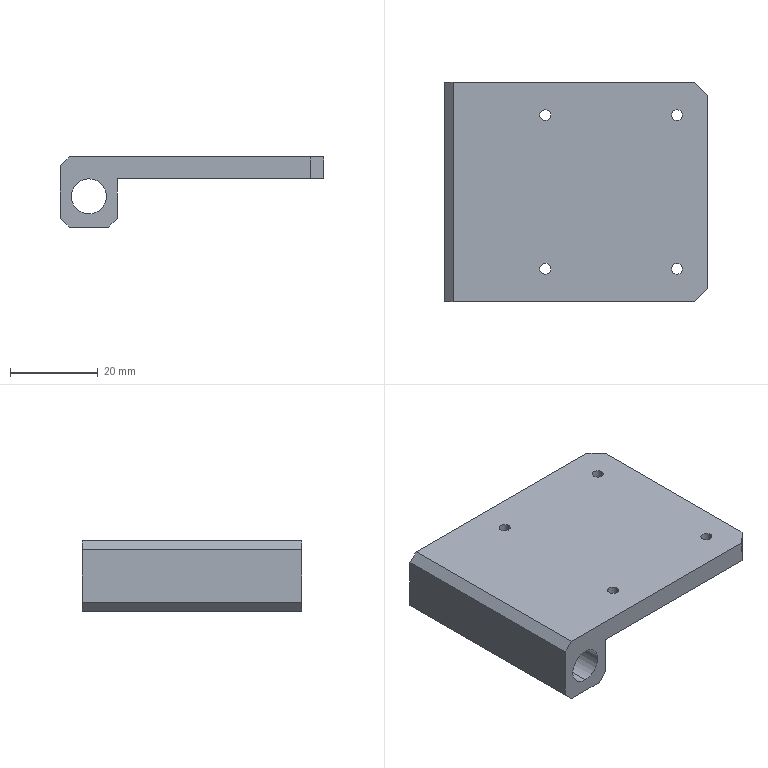Part | SolidWorks | features Chamfer 3, ICE 2, 3DProfileFeature 1, Extrusion 1, HoleWzd 1, LPattern 1 | 1 solid | 31 faces | box 60 x 50 x 16 mm | volume 19181 mm3 | plane 13 | cylinder 10 | cone 8 | commonest cylinder face diameters 2.5 x8 8 x2
STEP:
#1=CARTESIAN_POINT('',(24.25,42.5,-4.2));
#2=VERTEX_POINT('',#1);
#3=CARTESIAN_POINT('',(21.75,42.5,-4.2));
#4=VERTEX_POINT('',#3);
#5=CARTESIAN_POINT('',(23.,42.5,-4.2));
#6=DIRECTION('',(0.,0.,-1.));
#7=DIRECTION('',(1.,0.,0.));
#8=AXIS2_PLACEMENT_3D('',#5,#6,#7);
#9=CIRCLE('',#8,1.25);
#10=EDGE_CURVE('',#2,#4,#9,.T.);
#11=ORIENTED_EDGE('',*,*,#10,.F.);
#12=CARTESIAN_POINT('',(25.05,42.5,-5.));
#13=VERTEX_POINT('',#12);
#14=CARTESIAN_POINT('',(25.05,42.5,-5.));
#15=DIRECTION('',(0.7071,0.,-0.7071));
#16=VECTOR('',#15,1000.);
#17=LINE('',#14,#16);
#18=EDGE_CURVE('',#2,#13,#17,.T.);
#19=ORIENTED_EDGE('',*,*,#18,.T.);
#20=CARTESIAN_POINT('',(20.95,42.5,-5.));
#21=VERTEX_POINT('',#20);
#22=CARTESIAN_POINT('',(23.,42.5,-5.));
#23=DIRECTION('',(0.,0.,1.));
#24=DIRECTION('',(1.,0.,0.));
#25=AXIS2_PLACEMENT_3D('',#22,#23,#24);
#26=CIRCLE('',#25,2.05);
#27=EDGE_CURVE('',#21,#13,#26,.T.);
#28=ORIENTED_EDGE('',*,*,#27,.F.);
#29=CARTESIAN_POINT('',(20.95,42.5,-5.));
#30=DIRECTION('',(-0.7071,0.,-0.7071));
#31=VECTOR('',#30,1000.);
#32=LINE('',#29,#31);
#33=EDGE_CURVE('',#4,#21,#32,.T.);
#34=ORIENTED_EDGE('',*,*,#33,.F.);
#35=EDGE_LOOP('',(#11,#19,#28,#34));
#36=FACE_OUTER_BOUND('',#35,.T.);
#37=CARTESIAN_POINT('',(23.,42.5,-5.));
#38=DIRECTION('',(0.,0.,-1.));
#39=DIRECTION('',(-1.,0.,0.));
#40=AXIS2_PLACEMENT_3D('',#37,#38,#39);
#41=CONICAL_SURFACE('',#40,2.05,0.7854);
#42=ADVANCED_FACE('',(#36),#41,.F.);
#43=CARTESIAN_POINT('',(54.25,42.5,-4.2));
#44=VERTEX_POINT('',#43);
#45=CARTESIAN_POINT('',(51.75,42.5,-4.2));
#46=VERTEX_POINT('',#45);
#47=CARTESIAN_POINT('',(53.,42.5,-4.2));
#48=DIRECTION('',(0.,0.,-1.));
#49=DIRECTION('',(1.,0.,0.));
#50=AXIS2_PLACEMENT_3D('',#47,#48,#49);
#51=CIRCLE('',#50,1.25);
#52=EDGE_CURVE('',#44,#46,#51,.T.);
#53=ORIENTED_EDGE('',*,*,#52,.F.);
#54=CARTESIAN_POINT('',(55.05,42.5,-5.));
#55=VERTEX_POINT('',#54);
#56=CARTESIAN_POINT('',(55.05,42.5,-5.));
#57=DIRECTION('',(0.7071,0.,-0.7071));
#58=VECTOR('',#57,1000.);
#59=LINE('',#56,#58);
#60=EDGE_CURVE('',#44,#55,#59,.T.);
#61=ORIENTED_EDGE('',*,*,#60,.T.);
#62=CARTESIAN_POINT('',(50.95,42.5,-5.));
#63=VERTEX_POINT('',#62);
#64=CARTESIAN_POINT('',(53.,42.5,-5.));
#65=DIRECTION('',(0.,0.,1.));
#66=DIRECTION('',(1.,0.,0.));
#67=AXIS2_PLACEMENT_3D('',#64,#65,#66);
#68=CIRCLE('',#67,2.05);
#69=EDGE_CURVE('',#63,#55,#68,.T.);
#70=ORIENTED_EDGE('',*,*,#69,.F.);
#71=CARTESIAN_POINT('',(50.95,42.5,-5.));
#72=DIRECTION('',(-0.7071,0.,-0.7071));
#73=VECTOR('',#72,1000.);
#74=LINE('',#71,#73);
#75=EDGE_CURVE('',#46,#63,#74,.T.);
#76=ORIENTED_EDGE('',*,*,#75,.F.);
#77=EDGE_LOOP('',(#53,#61,#70,#76));
#78=FACE_OUTER_BOUND('',#77,.T.);
#79=CARTESIAN_POINT('',(53.,42.5,-5.));
#80=DIRECTION('',(0.,0.,-1.));
#81=DIRECTION('',(-1.,0.,0.));
#82=AXIS2_PLACEMENT_3D('',#79,#80,#81);
#83=CONICAL_SURFACE('',#82,2.05,0.7854);
#84=ADVANCED_FACE('',(#78),#83,.F.);
#85=CARTESIAN_POINT('',(24.25,7.5,-4.2));
#86=VERTEX_POINT('',#85);
#87=CARTESIAN_POINT('',(21.75,7.5,-4.2));
#88=VERTEX_POINT('',#87);
#89=CARTESIAN_POINT('',(23.,7.5,-4.2));
#90=DIRECTION('',(0.,0.,-1.));
#91=DIRECTION('',(1.,0.,0.));
#92=AXIS2_PLACEMENT_3D('',#89,#90,#91);
#93=CIRCLE('',#92,1.25);
#94=EDGE_CURVE('',#86,#88,#93,.T.);
#95=ORIENTED_EDGE('',*,*,#94,.F.);
#96=CARTESIAN_POINT('',(25.05,7.5,-5.));
#97=VERTEX_POINT('',#96);
#98=CARTESIAN_POINT('',(25.05,7.5,-5.));
#99=DIRECTION('',(0.7071,0.,-0.7071));
#100=VECTOR('',#99,1000.);
#101=LINE('',#98,#100);
#102=EDGE_CURVE('',#86,#97,#101,.T.);
#103=ORIENTED_EDGE('',*,*,#102,.T.);
#104=CARTESIAN_POINT('',(20.95,7.5,-5.));
#105=VERTEX_POINT('',#104);
#106=CARTESIAN_POINT('',(23.,7.5,-5.));
#107=DIRECTION('',(0.,0.,1.));
#108=DIRECTION('',(1.,0.,0.));
#109=AXIS2_PLACEMENT_3D('',#106,#107,#108);
#110=CIRCLE('',#109,2.05);
#111=EDGE_CURVE('',#105,#97,#110,.T.);
#112=ORIENTED_EDGE('',*,*,#111,.F.);
#113=CARTESIAN_POINT('',(20.95,7.5,-5.));
#114=DIRECTION('',(-0.7071,0.,-0.7071));
#115=VECTOR('',#114,1000.);
#116=LINE('',#113,#115);
#117=EDGE_CURVE('',#88,#105,#116,.T.);
#118=ORIENTED_EDGE('',*,*,#117,.F.);
#119=EDGE_LOOP('',(#95,#103,#112,#118));
#120=FACE_OUTER_BOUND('',#119,.T.);
#121=CARTESIAN_POINT('',(23.,7.5,-5.));
#122=DIRECTION('',(0.,0.,-1.));
#123=DIRECTION('',(-1.,0.,0.));
#124=AXIS2_PLACEMENT_3D('',#121,#122,#123);
#125=CONICAL_SURFACE('',#124,2.05,0.7854);
#126=ADVANCED_FACE('',(#120),#125,.F.);
#127=CARTESIAN_POINT('',(54.25,7.5,-4.2));
#128=VERTEX_POINT('',#127);
#129=CARTESIAN_POINT('',(51.75,7.5,-4.2));
#130=VERTEX_POINT('',#129);
#131=CARTESIAN_POINT('',(53.,7.5,-4.2));
#132=DIRECTION('',(0.,0.,-1.));
#133=DIRECTION('',(1.,0.,0.));
#134=AXIS2_PLACEMENT_3D('',#131,#132,#133);
#135=CIRCLE('',#134,1.25);
#136=EDGE_CURVE('',#128,#130,#135,.T.);
#137=ORIENTED_EDGE('',*,*,#136,.F.);
#138=CARTESIAN_POINT('',(55.05,7.5,-5.));
#139=VERTEX_POINT('',#138);
#140=CARTESIAN_POINT('',(55.05,7.5,-5.));
#141=DIRECTION('',(0.7071,0.,-0.7071));
#142=VECTOR('',#141,1000.);
#143=LINE('',#140,#142);
#144=EDGE_CURVE('',#128,#139,#143,.T.);
#145=ORIENTED_EDGE('',*,*,#144,.T.);
#146=CARTESIAN_POINT('',(50.95,7.5,-5.));
#147=VERTEX_POINT('',#146);
#148=CARTESIAN_POINT('',(53.,7.5,-5.));
#149=DIRECTION('',(0.,0.,1.));
#150=DIRECTION('',(1.,0.,0.));
#151=AXIS2_PLACEMENT_3D('',#148,#149,#150);
#152=CIRCLE('',#151,2.05);
#153=EDGE_CURVE('',#147,#139,#152,.T.);
#154=ORIENTED_EDGE('',*,*,#153,.F.);
#155=CARTESIAN_POINT('',(50.95,7.5,-5.));
#156=DIRECTION('',(-0.7071,0.,-0.7071));
#157=VECTOR('',#156,1000.);
#158=LINE('',#155,#157);
#159=EDGE_CURVE('',#130,#147,#158,.T.);
#160=ORIENTED_EDGE('',*,*,#159,.F.);
#161=EDGE_LOOP('',(#137,#145,#154,#160));
#162=FACE_OUTER_BOUND('',#161,.T.);
#163=CARTESIAN_POINT('',(53.,7.5,-5.));
#164=DIRECTION('',(0.,0.,-1.));
#165=DIRECTION('',(-1.,0.,0.));
#166=AXIS2_PLACEMENT_3D('',#163,#164,#165);
#167=CONICAL_SURFACE('',#166,2.05,0.7854);
#168=ADVANCED_FACE('',(#162),#167,.F.);
#169=ORIENTED_EDGE('',*,*,#10,.T.);
#170=CARTESIAN_POINT('',(21.75,42.5,0.));
#171=VERTEX_POINT('',#170);
#172=CARTESIAN_POINT('',(21.75,42.5,0.));
#173=DIRECTION('',(0.,0.,1.));
#174=VECTOR('',#173,1000.);
#175=LINE('',#172,#174);
#176=EDGE_CURVE('',#4,#171,#175,.T.);
#177=ORIENTED_EDGE('',*,*,#176,.T.);
#178=CARTESIAN_POINT('',(24.25,42.5,0.));
#179=VERTEX_POINT('',#178);
#180=CARTESIAN_POINT('',(23.,42.5,0.));
#181=DIRECTION('',(0.,0.,1.));
#182=DIRECTION('',(1.,0.,0.));
#183=AXIS2_PLACEMENT_3D('',#180,#181,#182);
#184=CIRCLE('',#183,1.25);
#185=EDGE_CURVE('',#171,#179,#184,.T.);
#186=ORIENTED_EDGE('',*,*,#185,.T.);
#187=CARTESIAN_POINT('',(24.25,42.5,0.));
#188=DIRECTION('',(0.,0.,1.));
#189=VECTOR('',#188,1000.);
#190=LINE('',#187,#189);
#191=EDGE_CURVE('',#2,#179,#190,.T.);
#192=ORIENTED_EDGE('',*,*,#191,.F.);
#193=EDGE_LOOP('',(#169,#177,#186,#192));
#194=FACE_OUTER_BOUND('',#193,.T.);
#195=CARTESIAN_POINT('',(23.,42.5,0.));
#196=DIRECTION('',(0.,0.,1.));
#197=DIRECTION('',(1.,0.,0.));
#198=AXIS2_PLACEMENT_3D('',#195,#196,#197);
#199=CYLINDRICAL_SURFACE('',#198,1.25);
#200=ADVANCED_FACE('',(#194),#199,.F.);
#201=ORIENTED_EDGE('',*,*,#52,.T.);
#202=CARTESIAN_POINT('',(51.75,42.5,0.));
#203=VERTEX_POINT('',#202);
#204=CARTESIAN_POINT('',(51.75,42.5,0.));
#205=DIRECTION('',(0.,0.,1.));
#206=VECTOR('',#205,1000.);
#207=LINE('',#204,#206);
#208=EDGE_CURVE('',#46,#203,#207,.T.);
#209=ORIENTED_EDGE('',*,*,#208,.T.);
#210=CARTESIAN_POINT('',(54.25,42.5,0.));
#211=VERTEX_POINT('',#210);
#212=CARTESIAN_POINT('',(53.,42.5,0.));
#213=DIRECTION('',(0.,0.,1.));
#214=DIRECTION('',(1.,0.,0.));
#215=AXIS2_PLACEMENT_3D('',#212,#213,#214);
#216=CIRCLE('',#215,1.25);
#217=EDGE_CURVE('',#203,#211,#216,.T.);
#218=ORIENTED_EDGE('',*,*,#217,.T.);
#219=CARTESIAN_POINT('',(54.25,42.5,0.));
#220=DIRECTION('',(0.,0.,1.));
#221=VECTOR('',#220,1000.);
#222=LINE('',#219,#221);
#223=EDGE_CURVE('',#44,#211,#222,.T.);
#224=ORIENTED_EDGE('',*,*,#223,.F.);
#225=EDGE_LOOP('',(#201,#209,#218,#224));
#226=FACE_OUTER_BOUND('',#225,.T.);
#227=CARTESIAN_POINT('',(53.,42.5,0.));
#228=DIRECTION('',(0.,0.,1.));
#229=DIRECTION('',(1.,0.,0.));
#230=AXIS2_PLACEMENT_3D('',#227,#228,#229);
#231=CYLINDRICAL_SURFACE('',#230,1.25);
#232=ADVANCED_FACE('',(#226),#231,.F.);
#233=ORIENTED_EDGE('',*,*,#136,.T.);
#234=CARTESIAN_POINT('',(51.75,7.5,0.));
#235=VERTEX_POINT('',#234);
#236=CARTESIAN_POINT('',(51.75,7.5,0.));
#237=DIRECTION('',(0.,0.,1.));
#238=VECTOR('',#237,1000.);
#239=LINE('',#236,#238);
#240=EDGE_CURVE('',#130,#235,#239,.T.);
#241=ORIENTED_EDGE('',*,*,#240,.T.);
#242=CARTESIAN_POINT('',(54.25,7.5,0.));
#243=VERTEX_POINT('',#242);
#244=CARTESIAN_POINT('',(53.,7.5,0.));
#245=DIRECTION('',(0.,0.,1.));
#246=DIRECTION('',(1.,0.,0.));
#247=AXIS2_PLACEMENT_3D('',#244,#245,#246);
#248=CIRCLE('',#247,1.25);
#249=EDGE_CURVE('',#235,#243,#248,.T.);
#250=ORIENTED_EDGE('',*,*,#249,.T.);
#251=CARTESIAN_POINT('',(54.25,7.5,0.));
#252=DIRECTION('',(0.,0.,1.));
#253=VECTOR('',#252,1000.);
#254=LINE('',#251,#253);
#255=EDGE_CURVE('',#128,#243,#254,.T.);
#256=ORIENTED_EDGE('',*,*,#255,.F.);
#257=EDGE_LOOP('',(#233,#241,#250,#256));
#258=FACE_OUTER_BOUND('',#257,.T.);
#259=CARTESIAN_POINT('',(53.,7.5,0.));
#260=DIRECTION('',(0.,0.,1.));
#261=DIRECTION('',(1.,0.,0.));
#262=AXIS2_PLACEMENT_3D('',#259,#260,#261);
#263=CYLINDRICAL_SURFACE('',#262,1.25);
#264=ADVANCED_FACE('',(#258),#263,.F.);
#265=ORIENTED_EDGE('',*,*,#94,.T.);
#266=CARTESIAN_POINT('',(21.75,7.5,0.));
#267=VERTEX_POINT('',#266);
#268=CARTESIAN_POINT('',(21.75,7.5,0.));
#269=DIRECTION('',(0.,0.,1.));
#270=VECTOR('',#269,1000.);
#271=LINE('',#268,#270);
#272=EDGE_CURVE('',#88,#267,#271,.T.);
#273=ORIENTED_EDGE('',*,*,#272,.T.);
#274=CARTESIAN_POINT('',(24.25,7.5,0.));
#275=VERTEX_POINT('',#274);
#276=CARTESIAN_POINT('',(23.,7.5,0.));
#277=DIRECTION('',(0.,0.,1.));
#278=DIRECTION('',(1.,0.,0.));
#279=AXIS2_PLACEMENT_3D('',#276,#277,#278);
#280=CIRCLE('',#279,1.25);
#281=EDGE_CURVE('',#267,#275,#280,.T.);
#282=ORIENTED_EDGE('',*,*,#281,.T.);
#283=CARTESIAN_POINT('',(24.25,7.5,0.));
#284=DIRECTION('',(0.,0.,1.));
#285=VECTOR('',#284,1000.);
#286=LINE('',#283,#285);
#287=EDGE_CURVE('',#86,#275,#286,.T.);
#288=ORIENTED_EDGE('',*,*,#287,.F.);
#289=EDGE_LOOP('',(#265,#273,#282,#288));
#290=FACE_OUTER_BOUND('',#289,.T.);
#291=CARTESIAN_POINT('',(23.,7.5,0.));
#292=DIRECTION('',(0.,0.,1.));
#293=DIRECTION('',(1.,0.,0.));
#294=AXIS2_PLACEMENT_3D('',#291,#292,#293);
#295=CYLINDRICAL_SURFACE('',#294,1.25);
#296=ADVANCED_FACE('',(#290),#295,.F.);
#297=CARTESIAN_POINT('',(6.5,0.,-5.));
#298=VERTEX_POINT('',#297);
#299=CARTESIAN_POINT('',(6.5,0.,-13.));
#300=VERTEX_POINT('',#299);
#301=CARTESIAN_POINT('',(6.5,0.,-9.));
#302=DIRECTION('',(0.,-1.,0.));
#303=DIRECTION('',(0.,0.,-1.));
#304=AXIS2_PLACEMENT_3D('',#301,#302,#303);
#305=CIRCLE('',#304,4.);
#306=EDGE_CURVE('',#298,#300,#305,.T.);
#307=ORIENTED_EDGE('',*,*,#306,.T.);
#308=CARTESIAN_POINT('',(6.5,50.,-13.));
#309=VERTEX_POINT('',#308);
#310=CARTESIAN_POINT('',(6.5,-10.,-13.));
#311=DIRECTION('',(0.,1.,0.));
#312=VECTOR('',#311,1000.);
#313=LINE('',#310,#312);
#314=EDGE_CURVE('',#300,#309,#313,.T.);
#315=ORIENTED_EDGE('',*,*,#314,.T.);
#316=CARTESIAN_POINT('',(6.5,50.,-5.));
#317=VERTEX_POINT('',#316);
#318=CARTESIAN_POINT('',(6.5,50.,-9.));
#319=DIRECTION('',(0.,1.,0.));
#320=DIRECTION('',(0.,0.,1.));
#321=AXIS2_PLACEMENT_3D('',#318,#319,#320);
#322=CIRCLE('',#321,4.);
#323=EDGE_CURVE('',#309,#317,#322,.T.);
#324=ORIENTED_EDGE('',*,*,#323,.T.);
#325=CARTESIAN_POINT('',(6.5,-10.,-5.));
#326=DIRECTION('',(0.,1.,0.));
#327=VECTOR('',#326,1000.);
#328=LINE('',#325,#327);
#329=EDGE_CURVE('',#298,#317,#328,.T.);
#330=ORIENTED_EDGE('',*,*,#329,.F.);
#331=EDGE_LOOP('',(#307,#315,#324,#330));
#332=FACE_OUTER_BOUND('',#331,.T.);
#333=CARTESIAN_POINT('',(6.5,-10.,-9.));
#334=DIRECTION('',(0.,1.,0.));
#335=DIRECTION('',(0.,0.,1.));
#336=AXIS2_PLACEMENT_3D('',#333,#334,#335);
#337=CYLINDRICAL_SURFACE('',#336,4.);
#338=ADVANCED_FACE('',(#332),#337,.F.);
#339=CARTESIAN_POINT('',(0.,0.,-14.));
#340=VERTEX_POINT('',#339);
#341=CARTESIAN_POINT('',(0.,0.,-2.));
#342=VERTEX_POINT('',#341);
#343=CARTESIAN_POINT('',(0.,0.,0.));
#344=DIRECTION('',(0.,0.,1.));
#345=VECTOR('',#344,1000.);
#346=LINE('',#343,#345);
#347=EDGE_CURVE('',#340,#342,#346,.T.);
#348=ORIENTED_EDGE('',*,*,#347,.T.);
#349=CARTESIAN_POINT('',(0.,50.,-2.));
#350=VERTEX_POINT('',#349);
#351=CARTESIAN_POINT('',(0.,50.,-2.));
#352=DIRECTION('',(0.,1.,0.));
#353=VECTOR('',#352,1000.);
#354=LINE('',#351,#353);
#355=EDGE_CURVE('',#342,#350,#354,.T.);
#356=ORIENTED_EDGE('',*,*,#355,.T.);
#357=CARTESIAN_POINT('',(0.,50.,-14.));
#358=VERTEX_POINT('',#357);
#359=CARTESIAN_POINT('',(0.,50.,0.));
#360=DIRECTION('',(0.,0.,1.));
#361=VECTOR('',#360,1000.);
#362=LINE('',#359,#361);
#363=EDGE_CURVE('',#358,#350,#362,.T.);
#364=ORIENTED_EDGE('',*,*,#363,.F.);
#365=CARTESIAN_POINT('',(0.,50.,-14.));
#366=DIRECTION('',(0.,-1.,0.));
#367=VECTOR('',#366,1000.);
#368=LINE('',#365,#367);
#369=EDGE_CURVE('',#358,#340,#368,.T.);
#370=ORIENTED_EDGE('',*,*,#369,.T.);
#371=EDGE_LOOP('',(#348,#356,#364,#370));
#372=FACE_OUTER_BOUND('',#371,.T.);
#373=CARTESIAN_POINT('',(0.,50.,0.));
#374=DIRECTION('',(1.,0.,0.));
#375=DIRECTION('',(0.,0.,-1.));
#376=AXIS2_PLACEMENT_3D('',#373,#374,#375);
#377=PLANE('',#376);
#378=ADVANCED_FACE('',(#372),#377,.F.);
#379=CARTESIAN_POINT('',(23.,42.5,0.));
#380=DIRECTION('',(0.,0.,1.));
#381=DIRECTION('',(1.,0.,0.));
#382=AXIS2_PLACEMENT_3D('',#379,#380,#381);
#383=CIRCLE('',#382,1.25);
#384=EDGE_CURVE('',#179,#171,#383,.T.);
#385=ORIENTED_EDGE('',*,*,#384,.F.);
#386=ORIENTED_EDGE('',*,*,#185,.F.);
#387=EDGE_LOOP('',(#385,#386));
#388=FACE_BOUND('',#387,.T.);
#389=CARTESIAN_POINT('',(53.,42.5,0.));
#390=DIRECTION('',(0.,0.,1.));
#391=DIRECTION('',(1.,0.,0.));
#392=AXIS2_PLACEMENT_3D('',#389,#390,#391);
#393=CIRCLE('',#392,1.25);
#394=EDGE_CURVE('',#211,#203,#393,.T.);
#395=ORIENTED_EDGE('',*,*,#394,.F.);
#396=ORIENTED_EDGE('',*,*,#217,.F.);
#397=EDGE_LOOP('',(#395,#396));
#398=FACE_BOUND('',#397,.T.);
#399=CARTESIAN_POINT('',(53.,7.5,0.));
#400=DIRECTION('',(0.,0.,1.));
#401=DIRECTION('',(1.,0.,0.));
#402=AXIS2_PLACEMENT_3D('',#399,#400,#401);
#403=CIRCLE('',#402,1.25);
#404=EDGE_CURVE('',#243,#235,#403,.T.);
#405=ORIENTED_EDGE('',*,*,#404,.F.);
#406=ORIENTED_EDGE('',*,*,#249,.F.);
#407=EDGE_LOOP('',(#405,#406));
#408=FACE_BOUND('',#407,.T.);
#409=CARTESIAN_POINT('',(23.,7.5,0.));
#410=DIRECTION('',(0.,0.,1.));
#411=DIRECTION('',(1.,0.,0.));
#412=AXIS2_PLACEMENT_3D('',#409,#410,#411);
#413=CIRCLE('',#412,1.25);
#414=EDGE_CURVE('',#275,#267,#413,.T.);
#415=ORIENTED_EDGE('',*,*,#414,.F.);
#416=ORIENTED_EDGE('',*,*,#281,.F.);
#417=EDGE_LOOP('',(#415,#416));
#418=FACE_BOUND('',#417,.T.);
#419=CARTESIAN_POINT('',(2.,0.,0.));
#420=VERTEX_POINT('',#419);
#421=CARTESIAN_POINT('',(57.,0.,0.));
#422=VERTEX_POINT('',#421);
#423=CARTESIAN_POINT('',(0.,0.,0.));
#424=DIRECTION('',(1.,0.,0.));
#425=VECTOR('',#424,1000.);
#426=LINE('',#423,#425);
#427=EDGE_CURVE('',#420,#422,#426,.T.);
#428=ORIENTED_EDGE('',*,*,#427,.T.);
#429=CARTESIAN_POINT('',(60.,3.,0.));
#430=VERTEX_POINT('',#429);
#431=CARTESIAN_POINT('',(60.,3.,0.));
#432=DIRECTION('',(0.7071,0.7071,0.));
#433=VECTOR('',#432,1000.);
#434=LINE('',#431,#433);
#435=EDGE_CURVE('',#422,#430,#434,.T.);
#436=ORIENTED_EDGE('',*,*,#435,.T.);
#437=CARTESIAN_POINT('',(60.,47.,0.));
#438=VERTEX_POINT('',#437);
#439=CARTESIAN_POINT('',(60.,50.,0.));
#440=DIRECTION('',(0.,-1.,0.));
#441=VECTOR('',#440,1000.);
#442=LINE('',#439,#441);
#443=EDGE_CURVE('',#438,#430,#442,.T.);
#444=ORIENTED_EDGE('',*,*,#443,.F.);
#445=CARTESIAN_POINT('',(57.,50.,0.));
#446=VERTEX_POINT('',#445);
#447=CARTESIAN_POINT('',(57.,50.,0.));
#448=DIRECTION('',(-0.7071,0.7071,0.));
#449=VECTOR('',#448,1000.);
#450=LINE('',#447,#449);
#451=EDGE_CURVE('',#438,#446,#450,.T.);
#452=ORIENTED_EDGE('',*,*,#451,.T.);
#453=CARTESIAN_POINT('',(2.,50.,0.));
#454=VERTEX_POINT('',#453);
#455=CARTESIAN_POINT('',(0.,50.,0.));
#456=DIRECTION('',(1.,0.,0.));
#457=VECTOR('',#456,1000.);
#458=LINE('',#455,#457);
#459=EDGE_CURVE('',#454,#446,#458,.T.);
#460=ORIENTED_EDGE('',*,*,#459,.F.);
#461=CARTESIAN_POINT('',(2.,50.,0.));
#462=DIRECTION('',(0.,-1.,0.));
#463=VECTOR('',#462,1000.);
#464=LINE('',#461,#463);
#465=EDGE_CURVE('',#454,#420,#464,.T.);
#466=ORIENTED_EDGE('',*,*,#465,.T.);
#467=EDGE_LOOP('',(#428,#436,#444,#452,#460,#466));
#468=FACE_OUTER_BOUND('',#467,.T.);
#469=CARTESIAN_POINT('',(0.,50.,0.));
#470=DIRECTION('',(0.,0.,-1.));
#471=DIRECTION('',(-1.,0.,0.));
#472=AXIS2_PLACEMENT_3D('',#469,#470,#471);
#473=PLANE('',#472);
#474=ADVANCED_FACE('',(#388,#398,#408,#418,#468),#473,.F.);
#475=ORIENTED_EDGE('',*,*,#443,.T.);
#476=CARTESIAN_POINT('',(60.,3.,-5.));
#477=VERTEX_POINT('',#476);
#478=CARTESIAN_POINT('',(60.,3.,-5.));
#479=DIRECTION('',(0.,0.,-1.));
#480=VECTOR('',#479,1000.);
#481=LINE('',#478,#480);
#482=EDGE_CURVE('',#430,#477,#481,.T.);
#483=ORIENTED_EDGE('',*,*,#482,.T.);
#484=CARTESIAN_POINT('',(60.,47.,-5.));
#485=VERTEX_POINT('',#484);
#486=CARTESIAN_POINT('',(60.,50.,-5.));
#487=DIRECTION('',(0.,-1.,0.));
#488=VECTOR('',#487,1000.);
#489=LINE('',#486,#488);
#490=EDGE_CURVE('',#485,#477,#489,.T.);
#491=ORIENTED_EDGE('',*,*,#490,.F.);
#492=CARTESIAN_POINT('',(60.,47.,0.));
#493=DIRECTION('',(0.,0.,1.));
#494=VECTOR('',#493,1000.);
#495=LINE('',#492,#494);
#496=EDGE_CURVE('',#485,#438,#495,.T.);
#497=ORIENTED_EDGE('',*,*,#496,.T.);
#498=EDGE_LOOP('',(#475,#483,#491,#497));
#499=FACE_OUTER_BOUND('',#498,.T.);
#500=CARTESIAN_POINT('',(60.,50.,0.));
#501=DIRECTION('',(-1.,0.,0.));
#502=DIRECTION('',(0.,0.,1.));
#503=AXIS2_PLACEMENT_3D('',#500,#501,#502);
#504=PLANE('',#503);
#505=ADVANCED_FACE('',(#499),#504,.F.);
#506=ORIENTED_EDGE('',*,*,#153,.T.);
#507=CARTESIAN_POINT('',(53.,7.5,-5.));
#508=DIRECTION('',(0.,0.,1.));
#509=DIRECTION('',(1.,0.,0.));
#510=AXIS2_PLACEMENT_3D('',#507,#508,#509);
#511=CIRCLE('',#510,2.05);
#512=EDGE_CURVE('',#139,#147,#511,.T.);
#513=ORIENTED_EDGE('',*,*,#512,.T.);
#514=EDGE_LOOP('',(#506,#513));
#515=FACE_BOUND('',#514,.T.);
#516=ORIENTED_EDGE('',*,*,#111,.T.);
#517=CARTESIAN_POINT('',(23.,7.5,-5.));
#518=DIRECTION('',(0.,0.,1.));
#519=DIRECTION('',(1.,0.,0.));
#520=AXIS2_PLACEMENT_3D('',#517,#518,#519);
#521=CIRCLE('',#520,2.05);
#522=EDGE_CURVE('',#97,#105,#521,.T.);
#523=ORIENTED_EDGE('',*,*,#522,.T.);
#524=EDGE_LOOP('',(#516,#523));
#525=FACE_BOUND('',#524,.T.);
#526=ORIENTED_EDGE('',*,*,#69,.T.);
#527=CARTESIAN_POINT('',(53.,42.5,-5.));
#528=DIRECTION('',(0.,0.,1.));
#529=DIRECTION('',(1.,0.,0.));
#530=AXIS2_PLACEMENT_3D('',#527,#528,#529);
#531=CIRCLE('',#530,2.05);
#532=EDGE_CURVE('',#55,#63,#531,.T.);
#533=ORIENTED_EDGE('',*,*,#532,.T.);
#534=EDGE_LOOP('',(#526,#533));
#535=FACE_BOUND('',#534,.T.);
#536=ORIENTED_EDGE('',*,*,#27,.T.);
#537=CARTESIAN_POINT('',(23.,42.5,-5.));
#538=DIRECTION('',(0.,0.,1.));
#539=DIRECTION('',(1.,0.,0.));
#540=AXIS2_PLACEMENT_3D('',#537,#538,#539);
#541=CIRCLE('',#540,2.05);
#542=EDGE_CURVE('',#13,#21,#541,.T.);
#543=ORIENTED_EDGE('',*,*,#542,.T.);
#544=EDGE_LOOP('',(#536,#543));
#545=FACE_BOUND('',#544,.T.);
#546=ORIENTED_EDGE('',*,*,#490,.T.);
#547=CARTESIAN_POINT('',(57.,0.,-5.));
#548=VERTEX_POINT('',#547);
#549=CARTESIAN_POINT('',(60.,3.,-5.));
#550=DIRECTION('',(-0.7071,-0.7071,0.));
#551=VECTOR('',#550,1000.);
#552=LINE('',#549,#551);
#553=EDGE_CURVE('',#477,#548,#552,.T.);
#554=ORIENTED_EDGE('',*,*,#553,.T.);
#555=CARTESIAN_POINT('',(13.,0.,-5.));
#556=VERTEX_POINT('',#555);
#557=CARTESIAN_POINT('',(60.,0.,-5.));
#558=DIRECTION('',(-1.,0.,0.));
#559=VECTOR('',#558,1000.);
#560=LINE('',#557,#559);
#561=EDGE_CURVE('',#548,#556,#560,.T.);
#562=ORIENTED_EDGE('',*,*,#561,.T.);
#563=CARTESIAN_POINT('',(13.,50.,-5.));
#564=VERTEX_POINT('',#563);
#565=CARTESIAN_POINT('',(13.,50.,-5.));
#566=DIRECTION('',(0.,-1.,0.));
#567=VECTOR('',#566,1000.);
#568=LINE('',#565,#567);
#569=EDGE_CURVE('',#564,#556,#568,.T.);
#570=ORIENTED_EDGE('',*,*,#569,.F.);
#571=CARTESIAN_POINT('',(57.,50.,-5.));
#572=VERTEX_POINT('',#571);
#573=CARTESIAN_POINT('',(60.,50.,-5.));
#574=DIRECTION('',(-1.,0.,0.));
#575=VECTOR('',#574,1000.);
#576=LINE('',#573,#575);
#577=EDGE_CURVE('',#572,#564,#576,.T.);
#578=ORIENTED_EDGE('',*,*,#577,.F.);
#579=CARTESIAN_POINT('',(57.,50.,-5.));
#580=DIRECTION('',(0.7071,-0.7071,0.));
#581=VECTOR('',#580,1000.);
#582=LINE('',#579,#581);
#583=EDGE_CURVE('',#572,#485,#582,.T.);
#584=ORIENTED_EDGE('',*,*,#583,.T.);
#585=EDGE_LOOP('',(#546,#554,#562,#570,#578,#584));
#586=FACE_OUTER_BOUND('',#585,.T.);
#587=CARTESIAN_POINT('',(60.,50.,-5.));
#588=DIRECTION('',(0.,0.,1.));
#589=DIRECTION('',(1.,0.,0.));
#590=AXIS2_PLACEMENT_3D('',#587,#588,#589);
#591=PLANE('',#590);
#592=ADVANCED_FACE('',(#515,#525,#535,#545,#586),#591,.F.);
#593=CARTESIAN_POINT('',(13.,0.,-14.));
#594=VERTEX_POINT('',#593);
#595=CARTESIAN_POINT('',(13.,0.,-16.));
#596=DIRECTION('',(0.,0.,-1.));
#597=VECTOR('',#596,1000.);
#598=LINE('',#595,#597);
#599=EDGE_CURVE('',#556,#594,#598,.T.);
#600=ORIENTED_EDGE('',*,*,#599,.T.);
#601=CARTESIAN_POINT('',(13.,50.,-14.));
#602=VERTEX_POINT('',#601);
#603=CARTESIAN_POINT('',(13.,50.,-14.));
#604=DIRECTION('',(0.,1.,0.));
#605=VECTOR('',#604,1000.);
#606=LINE('',#603,#605);
#607=EDGE_CURVE('',#594,#602,#606,.T.);
#608=ORIENTED_EDGE('',*,*,#607,.T.);
#609=CARTESIAN_POINT('',(13.,50.,-16.));
#610=DIRECTION('',(0.,0.,-1.));
#611=VECTOR('',#610,1000.);
#612=LINE('',#609,#611);
#613=EDGE_CURVE('',#564,#602,#612,.T.);
#614=ORIENTED_EDGE('',*,*,#613,.F.);
#615=ORIENTED_EDGE('',*,*,#569,.T.);
#616=EDGE_LOOP('',(#600,#608,#614,#615));
#617=FACE_OUTER_BOUND('',#616,.T.);
#618=CARTESIAN_POINT('',(13.,50.,-16.));
#619=DIRECTION('',(-1.,0.,0.));
#620=DIRECTION('',(0.,0.,1.));
#621=AXIS2_PLACEMENT_3D('',#618,#619,#620);
#622=PLANE('',#621);
#623=ADVANCED_FACE('',(#617),#622,.F.);
#624=CARTESIAN_POINT('',(11.,0.,-16.));
#625=VERTEX_POINT('',#624);
#626=CARTESIAN_POINT('',(2.,0.,-16.));
#627=VERTEX_POINT('',#626);
#628=CARTESIAN_POINT('',(0.,0.,-16.));
#629=DIRECTION('',(-1.,0.,0.));
#630=VECTOR('',#629,1000.);
#631=LINE('',#628,#630);
#632=EDGE_CURVE('',#625,#627,#631,.T.);
#633=ORIENTED_EDGE('',*,*,#632,.T.);
#634=CARTESIAN_POINT('',(2.,50.,-16.));
#635=VERTEX_POINT('',#634);
#636=CARTESIAN_POINT('',(2.,50.,-16.));
#637=DIRECTION('',(0.,1.,0.));
#638=VECTOR('',#637,1000.);
#639=LINE('',#636,#638);
#640=EDGE_CURVE('',#627,#635,#639,.T.);
#641=ORIENTED_EDGE('',*,*,#640,.T.);
#642=CARTESIAN_POINT('',(11.,50.,-16.));
#643=VERTEX_POINT('',#642);
#644=CARTESIAN_POINT('',(0.,50.,-16.));
#645=DIRECTION('',(-1.,0.,0.));
#646=VECTOR('',#645,1000.);
#647=LINE('',#644,#646);
#648=EDGE_CURVE('',#643,#635,#647,.T.);
#649=ORIENTED_EDGE('',*,*,#648,.F.);
#650=CARTESIAN_POINT('',(11.,50.,-16.));
#651=DIRECTION('',(0.,-1.,0.));
#652=VECTOR('',#651,1000.);
#653=LINE('',#650,#652);
#654=EDGE_CURVE('',#643,#625,#653,.T.);
#655=ORIENTED_EDGE('',*,*,#654,.T.);
#656=EDGE_LOOP('',(#633,#641,#649,#655));
#657=FACE_OUTER_BOUND('',#656,.T.);
#658=CARTESIAN_POINT('',(0.,50.,-16.));
#659=DIRECTION('',(0.,0.,1.));
#660=DIRECTION('',(1.,0.,0.));
#661=AXIS2_PLACEMENT_3D('',#658,#659,#660);
#662=PLANE('',#661);
#663=ADVANCED_FACE('',(#657),#662,.F.);
#664=CARTESIAN_POINT('',(6.5,50.,-9.));
#665=DIRECTION('',(0.,1.,0.));
#666=DIRECTION('',(0.,0.,1.));
#667=AXIS2_PLACEMENT_3D('',#664,#665,#666);
#668=CIRCLE('',#667,4.);
#669=EDGE_CURVE('',#317,#309,#668,.T.);
#670=ORIENTED_EDGE('',*,*,#669,.F.);
#671=ORIENTED_EDGE('',*,*,#323,.F.);
#672=EDGE_LOOP('',(#670,#671));
#673=FACE_BOUND('',#672,.T.);
#674=ORIENTED_EDGE('',*,*,#459,.T.);
#675=CARTESIAN_POINT('',(57.,50.,0.));
#676=DIRECTION('',(0.,0.,-1.));
#677=VECTOR('',#676,1000.);
#678=LINE('',#675,#677);
#679=EDGE_CURVE('',#446,#572,#678,.T.);
#680=ORIENTED_EDGE('',*,*,#679,.T.);
#681=ORIENTED_EDGE('',*,*,#577,.T.);
#682=ORIENTED_EDGE('',*,*,#613,.T.);
#683=CARTESIAN_POINT('',(11.,50.,-16.));
#684=DIRECTION('',(-0.7071,0.,-0.7071));
#685=VECTOR('',#684,1000.);
#686=LINE('',#683,#685);
#687=EDGE_CURVE('',#602,#643,#686,.T.);
#688=ORIENTED_EDGE('',*,*,#687,.T.);
#689=ORIENTED_EDGE('',*,*,#648,.T.);
#690=CARTESIAN_POINT('',(0.,50.,-14.));
#691=DIRECTION('',(-0.7071,0.,0.7071));
#692=VECTOR('',#691,1000.);
#693=LINE('',#690,#692);
#694=EDGE_CURVE('',#635,#358,#693,.T.);
#695=ORIENTED_EDGE('',*,*,#694,.T.);
#696=ORIENTED_EDGE('',*,*,#363,.T.);
#697=CARTESIAN_POINT('',(2.,50.,0.));
#698=DIRECTION('',(0.7071,0.,0.7071));
#699=VECTOR('',#698,1000.);
#700=LINE('',#697,#699);
#701=EDGE_CURVE('',#350,#454,#700,.T.);
#702=ORIENTED_EDGE('',*,*,#701,.T.);
#703=EDGE_LOOP('',(#674,#680,#681,#682,#688,#689,#695,#696,#702));
#704=FACE_OUTER_BOUND('',#703,.T.);
#705=CARTESIAN_POINT('',(0.,50.,0.));
#706=DIRECTION('',(0.,-1.,0.));
#707=DIRECTION('',(0.,0.,-1.));
#708=AXIS2_PLACEMENT_3D('',#705,#706,#707);
#709=PLANE('',#708);
#710=ADVANCED_FACE('',(#673,#704),#709,.F.);
#711=ORIENTED_EDGE('',*,*,#306,.F.);
#712=CARTESIAN_POINT('',(6.5,0.,-9.));
#713=DIRECTION('',(0.,-1.,0.));
#714=DIRECTION('',(0.,0.,-1.));
#715=AXIS2_PLACEMENT_3D('',#712,#713,#714);
#716=CIRCLE('',#715,4.);
#717=EDGE_CURVE('',#300,#298,#716,.T.);
#718=ORIENTED_EDGE('',*,*,#717,.F.);
#719=EDGE_LOOP('',(#711,#718));
#720=FACE_BOUND('',#719,.T.);
#721=ORIENTED_EDGE('',*,*,#561,.F.);
#722=CARTESIAN_POINT('',(57.,0.,0.));
#723=DIRECTION('',(0.,0.,1.));
#724=VECTOR('',#723,1000.);
#725=LINE('',#722,#724);
#726=EDGE_CURVE('',#548,#422,#725,.T.);
#727=ORIENTED_EDGE('',*,*,#726,.T.);
#728=ORIENTED_EDGE('',*,*,#427,.F.);
#729=CARTESIAN_POINT('',(1.,0.,-1.));
#730=DIRECTION('',(-0.7071,0.,-0.7071));
#731=VECTOR('',#730,1000.);
#732=LINE('',#729,#731);
#733=EDGE_CURVE('',#420,#342,#732,.T.);
#734=ORIENTED_EDGE('',*,*,#733,.T.);
#735=ORIENTED_EDGE('',*,*,#347,.F.);
#736=CARTESIAN_POINT('',(-7.,0.,-7.));
#737=DIRECTION('',(0.7071,0.,-0.7071));
#738=VECTOR('',#737,1000.);
#739=LINE('',#736,#738);
#740=EDGE_CURVE('',#340,#627,#739,.T.);
#741=ORIENTED_EDGE('',*,*,#740,.T.);
#742=ORIENTED_EDGE('',*,*,#632,.F.);
#743=CARTESIAN_POINT('',(13.5,0.,-13.5));
#744=DIRECTION('',(0.7071,0.,0.7071));
#745=VECTOR('',#744,1000.);
#746=LINE('',#743,#745);
#747=EDGE_CURVE('',#625,#594,#746,.T.);
#748=ORIENTED_EDGE('',*,*,#747,.T.);
#749=ORIENTED_EDGE('',*,*,#599,.F.);
#750=EDGE_LOOP('',(#721,#727,#728,#734,#735,#741,#742,#748,#749));
#751=FACE_OUTER_BOUND('',#750,.T.);
#752=CARTESIAN_POINT('',(0.,0.,0.));
#753=DIRECTION('',(0.,-1.,0.));
#754=DIRECTION('',(0.,0.,-1.));
#755=AXIS2_PLACEMENT_3D('',#752,#753,#754);
#756=PLANE('',#755);
#757=ADVANCED_FACE('',(#720,#751),#756,.T.);
#758=ORIENTED_EDGE('',*,*,#314,.F.);
#759=ORIENTED_EDGE('',*,*,#717,.T.);
#760=ORIENTED_EDGE('',*,*,#329,.T.);
#761=ORIENTED_EDGE('',*,*,#669,.T.);
#762=EDGE_LOOP('',(#758,#759,#760,#761));
#763=FACE_OUTER_BOUND('',#762,.T.);
#764=CARTESIAN_POINT('',(6.5,-10.,-9.));
#765=DIRECTION('',(0.,1.,0.));
#766=DIRECTION('',(0.,0.,1.));
#767=AXIS2_PLACEMENT_3D('',#764,#765,#766);
#768=CYLINDRICAL_SURFACE('',#767,4.);
#769=ADVANCED_FACE('',(#763),#768,.F.);
#770=ORIENTED_EDGE('',*,*,#701,.F.);
#771=ORIENTED_EDGE('',*,*,#355,.F.);
#772=ORIENTED_EDGE('',*,*,#733,.F.);
#773=ORIENTED_EDGE('',*,*,#465,.F.);
#774=EDGE_LOOP('',(#770,#771,#772,#773));
#775=FACE_OUTER_BOUND('',#774,.T.);
#776=CARTESIAN_POINT('',(2.,50.,0.));
#777=DIRECTION('',(0.7071,0.,-0.7071));
#778=DIRECTION('',(0.,-1.,0.));
#779=AXIS2_PLACEMENT_3D('',#776,#777,#778);
#780=PLANE('',#779);
#781=ADVANCED_FACE('',(#775),#780,.F.);
#782=ORIENTED_EDGE('',*,*,#694,.F.);
#783=ORIENTED_EDGE('',*,*,#640,.F.);
#784=ORIENTED_EDGE('',*,*,#740,.F.);
#785=ORIENTED_EDGE('',*,*,#369,.F.);
#786=EDGE_LOOP('',(#782,#783,#784,#785));
#787=FACE_OUTER_BOUND('',#786,.T.);
#788=CARTESIAN_POINT('',(0.,50.,-14.));
#789=DIRECTION('',(0.7071,0.,0.7071));
#790=DIRECTION('',(0.,-1.,0.));
#791=AXIS2_PLACEMENT_3D('',#788,#789,#790);
#792=PLANE('',#791);
#793=ADVANCED_FACE('',(#787),#792,.F.);
#794=ORIENTED_EDGE('',*,*,#687,.F.);
#795=ORIENTED_EDGE('',*,*,#607,.F.);
#796=ORIENTED_EDGE('',*,*,#747,.F.);
#797=ORIENTED_EDGE('',*,*,#654,.F.);
#798=EDGE_LOOP('',(#794,#795,#796,#797));
#799=FACE_OUTER_BOUND('',#798,.T.);
#800=CARTESIAN_POINT('',(11.,50.,-16.));
#801=DIRECTION('',(-0.7071,0.,0.7071));
#802=DIRECTION('',(0.,-1.,0.));
#803=AXIS2_PLACEMENT_3D('',#800,#801,#802);
#804=PLANE('',#803);
#805=ADVANCED_FACE('',(#799),#804,.F.);
#806=ORIENTED_EDGE('',*,*,#435,.F.);
#807=ORIENTED_EDGE('',*,*,#726,.F.);
#808=ORIENTED_EDGE('',*,*,#553,.F.);
#809=ORIENTED_EDGE('',*,*,#482,.F.);
#810=EDGE_LOOP('',(#806,#807,#808,#809));
#811=FACE_OUTER_BOUND('',#810,.T.);
#812=CARTESIAN_POINT('',(60.,3.,0.));
#813=DIRECTION('',(0.7071,-0.7071,0.));
#814=DIRECTION('',(0.,0.,1.));
#815=AXIS2_PLACEMENT_3D('',#812,#813,#814);
#816=PLANE('',#815);
#817=ADVANCED_FACE('',(#811),#816,.T.);
#818=ORIENTED_EDGE('',*,*,#451,.F.);
#819=ORIENTED_EDGE('',*,*,#496,.F.);
#820=ORIENTED_EDGE('',*,*,#583,.F.);
#821=ORIENTED_EDGE('',*,*,#679,.F.);
#822=EDGE_LOOP('',(#818,#819,#820,#821));
#823=FACE_OUTER_BOUND('',#822,.T.);
#824=CARTESIAN_POINT('',(57.,50.,0.));
#825=DIRECTION('',(-0.7071,-0.7071,0.));
#826=DIRECTION('',(0.,0.,-1.));
#827=AXIS2_PLACEMENT_3D('',#824,#825,#826);
#828=PLANE('',#827);
#829=ADVANCED_FACE('',(#823),#828,.F.);
#830=ORIENTED_EDGE('',*,*,#272,.F.);
#831=CARTESIAN_POINT('',(23.,7.5,-4.2));
#832=DIRECTION('',(0.,0.,-1.));
#833=DIRECTION('',(1.,0.,0.));
#834=AXIS2_PLACEMENT_3D('',#831,#832,#833);
#835=CIRCLE('',#834,1.25);
#836=EDGE_CURVE('',#88,#86,#835,.T.);
#837=ORIENTED_EDGE('',*,*,#836,.T.);
#838=ORIENTED_EDGE('',*,*,#287,.T.);
#839=ORIENTED_EDGE('',*,*,#414,.T.);
#840=EDGE_LOOP('',(#830,#837,#838,#839));
#841=FACE_OUTER_BOUND('',#840,.T.);
#842=CARTESIAN_POINT('',(23.,7.5,0.));
#843=DIRECTION('',(0.,0.,1.));
#844=DIRECTION('',(1.,0.,0.));
#845=AXIS2_PLACEMENT_3D('',#842,#843,#844);
#846=CYLINDRICAL_SURFACE('',#845,1.25);
#847=ADVANCED_FACE('',(#841),#846,.F.);
#848=ORIENTED_EDGE('',*,*,#240,.F.);
#849=CARTESIAN_POINT('',(53.,7.5,-4.2));
#850=DIRECTION('',(0.,0.,-1.));
#851=DIRECTION('',(1.,0.,0.));
#852=AXIS2_PLACEMENT_3D('',#849,#850,#851);
#853=CIRCLE('',#852,1.25);
#854=EDGE_CURVE('',#130,#128,#853,.T.);
#855=ORIENTED_EDGE('',*,*,#854,.T.);
#856=ORIENTED_EDGE('',*,*,#255,.T.);
#857=ORIENTED_EDGE('',*,*,#404,.T.);
#858=EDGE_LOOP('',(#848,#855,#856,#857));
#859=FACE_OUTER_BOUND('',#858,.T.);
#860=CARTESIAN_POINT('',(53.,7.5,0.));
#861=DIRECTION('',(0.,0.,1.));
#862=DIRECTION('',(1.,0.,0.));
#863=AXIS2_PLACEMENT_3D('',#860,#861,#862);
#864=CYLINDRICAL_SURFACE('',#863,1.25);
#865=ADVANCED_FACE('',(#859),#864,.F.);
#866=ORIENTED_EDGE('',*,*,#208,.F.);
#867=CARTESIAN_POINT('',(53.,42.5,-4.2));
#868=DIRECTION('',(0.,0.,-1.));
#869=DIRECTION('',(1.,0.,0.));
#870=AXIS2_PLACEMENT_3D('',#867,#868,#869);
#871=CIRCLE('',#870,1.25);
#872=EDGE_CURVE('',#46,#44,#871,.T.);
#873=ORIENTED_EDGE('',*,*,#872,.T.);
#874=ORIENTED_EDGE('',*,*,#223,.T.);
#875=ORIENTED_EDGE('',*,*,#394,.T.);
#876=EDGE_LOOP('',(#866,#873,#874,#875));
#877=FACE_OUTER_BOUND('',#876,.T.);
#878=CARTESIAN_POINT('',(53.,42.5,0.));
#879=DIRECTION('',(0.,0.,1.));
#880=DIRECTION('',(1.,0.,0.));
#881=AXIS2_PLACEMENT_3D('',#878,#879,#880);
#882=CYLINDRICAL_SURFACE('',#881,1.25);
#883=ADVANCED_FACE('',(#877),#882,.F.);
#884=ORIENTED_EDGE('',*,*,#176,.F.);
#885=CARTESIAN_POINT('',(23.,42.5,-4.2));
#886=DIRECTION('',(0.,0.,-1.));
#887=DIRECTION('',(1.,0.,0.));
#888=AXIS2_PLACEMENT_3D('',#885,#886,#887);
#889=CIRCLE('',#888,1.25);
#890=EDGE_CURVE('',#4,#2,#889,.T.);
#891=ORIENTED_EDGE('',*,*,#890,.T.);
#892=ORIENTED_EDGE('',*,*,#191,.T.);
#893=ORIENTED_EDGE('',*,*,#384,.T.);
#894=EDGE_LOOP('',(#884,#891,#892,#893));
#895=FACE_OUTER_BOUND('',#894,.T.);
#896=CARTESIAN_POINT('',(23.,42.5,0.));
#897=DIRECTION('',(0.,0.,1.));
#898=DIRECTION('',(1.,0.,0.));
#899=AXIS2_PLACEMENT_3D('',#896,#897,#898);
#900=CYLINDRICAL_SURFACE('',#899,1.25);
#901=ADVANCED_FACE('',(#895),#900,.F.);
#902=ORIENTED_EDGE('',*,*,#144,.F.);
#903=ORIENTED_EDGE('',*,*,#854,.F.);
#904=ORIENTED_EDGE('',*,*,#159,.T.);
#905=ORIENTED_EDGE('',*,*,#512,.F.);
#906=EDGE_LOOP('',(#902,#903,#904,#905));
#907=FACE_OUTER_BOUND('',#906,.T.);
#908=CARTESIAN_POINT('',(53.,7.5,-5.));
#909=DIRECTION('',(0.,0.,-1.));
#910=DIRECTION('',(-1.,0.,0.));
#911=AXIS2_PLACEMENT_3D('',#908,#909,#910);
#912=CONICAL_SURFACE('',#911,2.05,0.7854);
#913=ADVANCED_FACE('',(#907),#912,.F.);
#914=ORIENTED_EDGE('',*,*,#102,.F.);
#915=ORIENTED_EDGE('',*,*,#836,.F.);
#916=ORIENTED_EDGE('',*,*,#117,.T.);
#917=ORIENTED_EDGE('',*,*,#522,.F.);
#918=EDGE_LOOP('',(#914,#915,#916,#917));
#919=FACE_OUTER_BOUND('',#918,.T.);
#920=CARTESIAN_POINT('',(23.,7.5,-5.));
#921=DIRECTION('',(0.,0.,-1.));
#922=DIRECTION('',(-1.,0.,0.));
#923=AXIS2_PLACEMENT_3D('',#920,#921,#922);
#924=CONICAL_SURFACE('',#923,2.05,0.7854);
#925=ADVANCED_FACE('',(#919),#924,.F.);
#926=ORIENTED_EDGE('',*,*,#60,.F.);
#927=ORIENTED_EDGE('',*,*,#872,.F.);
#928=ORIENTED_EDGE('',*,*,#75,.T.);
#929=ORIENTED_EDGE('',*,*,#532,.F.);
#930=EDGE_LOOP('',(#926,#927,#928,#929));
#931=FACE_OUTER_BOUND('',#930,.T.);
#932=CARTESIAN_POINT('',(53.,42.5,-5.));
#933=DIRECTION('',(0.,0.,-1.));
#934=DIRECTION('',(-1.,0.,0.));
#935=AXIS2_PLACEMENT_3D('',#932,#933,#934);
#936=CONICAL_SURFACE('',#935,2.05,0.7854);
#937=ADVANCED_FACE('',(#931),#936,.F.);
#938=ORIENTED_EDGE('',*,*,#18,.F.);
#939=ORIENTED_EDGE('',*,*,#890,.F.);
#940=ORIENTED_EDGE('',*,*,#33,.T.);
#941=ORIENTED_EDGE('',*,*,#542,.F.);
#942=EDGE_LOOP('',(#938,#939,#940,#941));
#943=FACE_OUTER_BOUND('',#942,.T.);
#944=CARTESIAN_POINT('',(23.,42.5,-5.));
#945=DIRECTION('',(0.,0.,-1.));
#946=DIRECTION('',(-1.,0.,0.));
#947=AXIS2_PLACEMENT_3D('',#944,#945,#946);
#948=CONICAL_SURFACE('',#947,2.05,0.7854);
#949=ADVANCED_FACE('',(#943),#948,.F.);
#950=CLOSED_SHELL('',(#42,#84,#126,#168,#200,#232,#264,#296,#338,#378,#474,#505,#592,#623,#663,#710,#757,#769,#781,#793,#805,#817,#829,#847,#865,#883,#901,#913,#925,#937,#949));
#951=MANIFOLD_SOLID_BREP('',#950);
#952=CARTESIAN_POINT('',(0.,0.,0.));
#953=DIRECTION('',(0.,0.,1.));
#954=DIRECTION('',(1.,0.,0.));
#955=AXIS2_PLACEMENT_3D('',#952,#953,#954);
#956=(LENGTH_UNIT()NAMED_UNIT(*)SI_UNIT(.MILLI.,.METRE.));
#957=UNCERTAINTY_MEASURE_WITH_UNIT(LENGTH_MEASURE(0.00001),#956,'','');
#958=(NAMED_UNIT(*)PLANE_ANGLE_UNIT()SI_UNIT($,.RADIAN.));
#959=(NAMED_UNIT(*)SI_UNIT($,.STERADIAN.)SOLID_ANGLE_UNIT());
#960=(GEOMETRIC_REPRESENTATION_CONTEXT(3)GLOBAL_UNCERTAINTY_ASSIGNED_CONTEXT((#957))GLOBAL_UNIT_ASSIGNED_CONTEXT((#956,#958,#959))REPRESENTATION_CONTEXT('',''));
#961=ADVANCED_BREP_SHAPE_REPRESENTATION('',(#951,#955),#960);